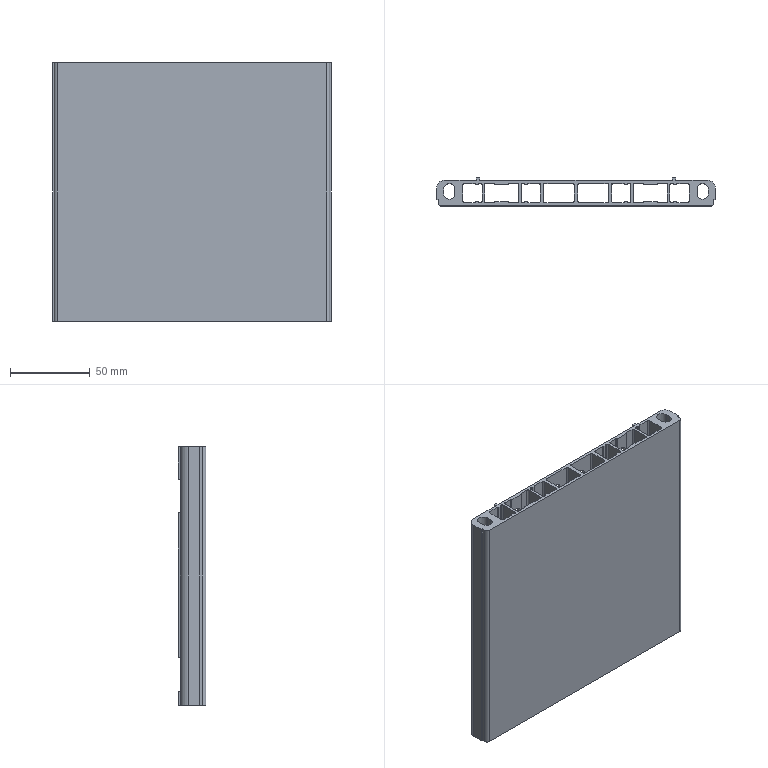Part | NX | features BREP 1 | 1 solid | 216 faces | box 175 x 17.5 x 162.4 mm | volume 177412 mm3 | cylinder 114 | plane 102 | commonest cylinder face diameters 0.6 x56 2 x32 6.5 x12 12 x6 7 x4 4 x2